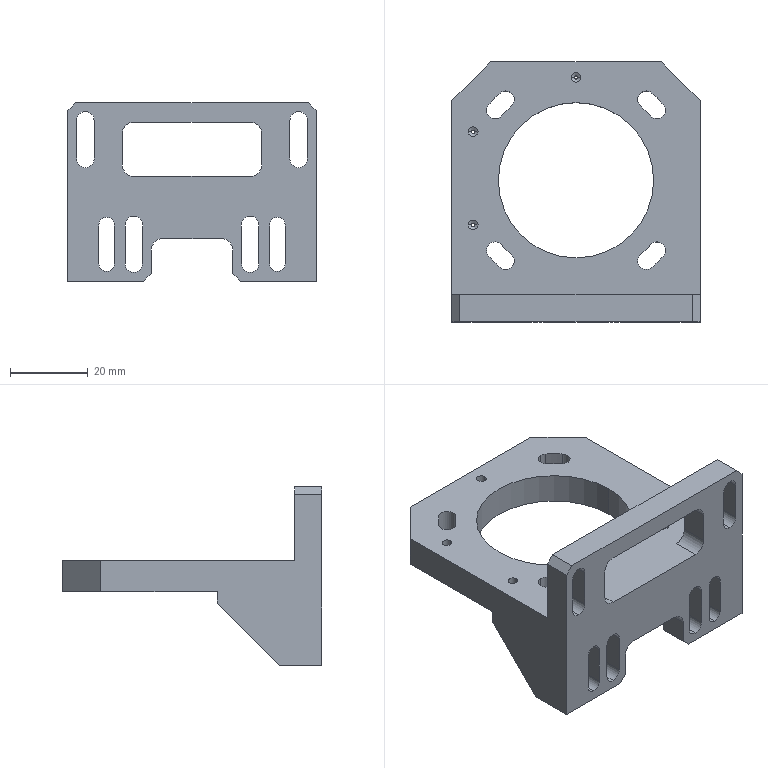NC program | NX | posted with a generic post | part box 64 x 67 x 46 mm
Lines 8580 to 8734 of 8734:
(PLANAR_MILL_COPY_COPY_COPY_1 , TOOL : D6A45)
N17134 T07 M6
N17136 G54
N17138 G17 G0 G90 X-15.15 Y14.77 B0. C0. S7500 M3
N17140 G43 Z30. H7
N17142 Z0.5
N17144 G94 G1 Z-1. F1250.
N17146 X-15.85 Y14.366
N17148 G3 X-16.35 Y13.5 R1.
N17150 G1 Y8.5
N17152 G3 X-15. Y7.15 R1.35
N17154 X-13.65 Y8.5 R1.35
N17156 G1 Y18.5
N17158 G3 X-15. Y19.85 R1.35
N17160 X-16.35 Y18.5 R1.35
N17162 G1 Y13.5
N17164 G3 X-15.85 Y12.634 R1.
N17166 G1 X-15.15 Y12.23
N17168 Z0.5
N17170 G0 Z30.
N17172 X-22.935 Y19.055
N17174 Z0.5
N17176 G1 X-23.1 Y18.759 Z0.409
N17178 Y13.5 Z-1.
N17180 Y8.5
N17182 G3 X-22. Y7.4 R1.1
N17184 X-20.9 Y8.5 R1.1
N17186 G1 Y18.5
N17188 G3 X-22. Y19.6 R1.1
N17190 X-23.1 Y18.5 R1.1
N17192 G1 Y13.5
N17194 G3 X-22.6 Y12.634 R1.
N17196 G1 Z0.5
N17198 G0 Z30.
N17200 X-27.65 Y-12.23
N17202 Z0.5
N17204 G1 Z-1.
N17206 X-28.35 Y-12.634
N17208 G3 X-28.85 Y-13.5 R1.
N17210 G1 Y-18.5
N17212 G3 X-27.5 Y-19.85 R1.35
N17214 X-26.15 Y-18.5 R1.35
N17216 G1 Y-8.5
N17218 G3 X-27.5 Y-7.15 R1.35
N17220 X-28.85 Y-8.5 R1.35
N17222 G1 Y-13.5
N17224 G3 X-28.35 Y-14.366 R1.
N17226 G1 X-27.65 Y-14.77
N17228 Z0.5
N17230 G0 Z30.
N17232 X-1.27 Y-15.9
N17234 Z0.5
N17236 G1 Z-1.
N17238 X-0.866 Y-16.6
N17240 G3 X0. Y-17.1 R1.
N17242 G1 X15.
N17244 G3 X17.1 Y-15. R2.1
N17246 G1 Y-7.
N17248 G3 X15. Y-4.9 R2.1
N17250 G1 X-15.
N17252 G3 X-17.1 Y-7. R2.1
N17254 G1 Y-15.
N17256 G3 X-15. Y-17.1 R2.1
N17258 G1 X0.
N17260 G3 X0.866 Y-16.6 R1.
N17262 G1 X1.27 Y-15.9
N17264 Z0.5
N17266 G0 Z30.
N17268 X27.65 Y-14.77
N17270 Z0.5
N17272 G1 Z-1.
N17274 X28.35 Y-14.366
N17276 G3 X28.85 Y-13.5 R1.
N17278 G1 Y-8.5
N17280 G3 X27.5 Y-7.15 R1.35
N17282 X26.15 Y-8.5 R1.35
N17284 G1 Y-18.5
N17286 G3 X27.5 Y-19.85 R1.35
N17288 X28.85 Y-18.5 R1.35
N17290 G1 Y-13.5
N17292 G3 X28.35 Y-12.634 R1.
N17294 G1 X27.65 Y-12.23
N17296 Z0.5
N17298 G0 Z30.
N17300 X22.935 Y7.945
N17302 Z0.5
N17304 G1 X23.1 Y8.241 Z0.409
N17306 Y13.5 Z-1.
N17308 Y18.5
N17310 G3 X22. Y19.6 R1.1
N17312 X20.9 Y18.5 R1.1
N17314 G1 Y8.5
N17316 G3 X22. Y7.4 R1.1
N17318 X23.1 Y8.5 R1.1
N17320 G1 Y13.5
N17322 G3 X22.6 Y14.366 R1.
N17324 G1 Z0.5
N17326 G0 Z30.
N17328 X15.15 Y12.23
N17330 Z0.5
N17332 G1 Z-1.
N17334 X15.85 Y12.634
N17336 G3 X16.35 Y13.5 R1.
N17338 G1 Y18.5
N17340 G3 X15. Y19.85 R1.35
N17342 X13.65 Y18.5 R1.35
N17344 G1 Y8.5
N17346 G3 X15. Y7.15 R1.35
N17348 X16.35 Y8.5 R1.35
N17350 G1 Y13.5
N17352 G3 X15.85 Y14.366 R1.
N17354 G1 X15.15 Y14.77
N17356 Z0.5
N17358 G0 Z30.
N17360 M5
(刀补 , TOOL : D3)
N17362 T03 M6
N17364 G54
N17366 G17 G0 G90 X21.567 Y18.598 B0. C0. S7500 M3
N17368 G43 Z30. H3
N17370 Z1.
N17372 G94 G1 Z-7. F1000.
N17374 G41 X21.55 Y18.5 D3
N17376 Y8.5
N17378 G3 X22. Y8.05 R0.45
N17380 X22.45 Y8.5 R0.45
N17382 G1 Y18.5
N17384 G3 X22. Y18.95 R0.45
N17386 X21.55 Y18.5 R0.45
N17388 X21.7 Y18.24 R0.3
N17390 G40
N17392 G1 X21.794 Y18.206
N17394 Z-6.
N17396 G0 Z30.
N17398 X-22.433 Y18.598
N17400 Z1.
N17402 G1 Z-7.
N17404 G41 X-22.45 Y18.5
N17406 Y8.5
N17408 G3 X-22. Y8.05 R0.45
N17410 X-21.55 Y8.5 R0.45
N17412 G1 Y18.5
N17414 G3 X-22. Y18.95 R0.45
N17416 X-22.45 Y18.5 R0.45
N17418 X-22.3 Y18.24 R0.3
N17420 G40
N17422 G1 X-22.206 Y18.206
N17424 Z-6.
N17426 G0 Z30.
N17428 M5
N17430 M2